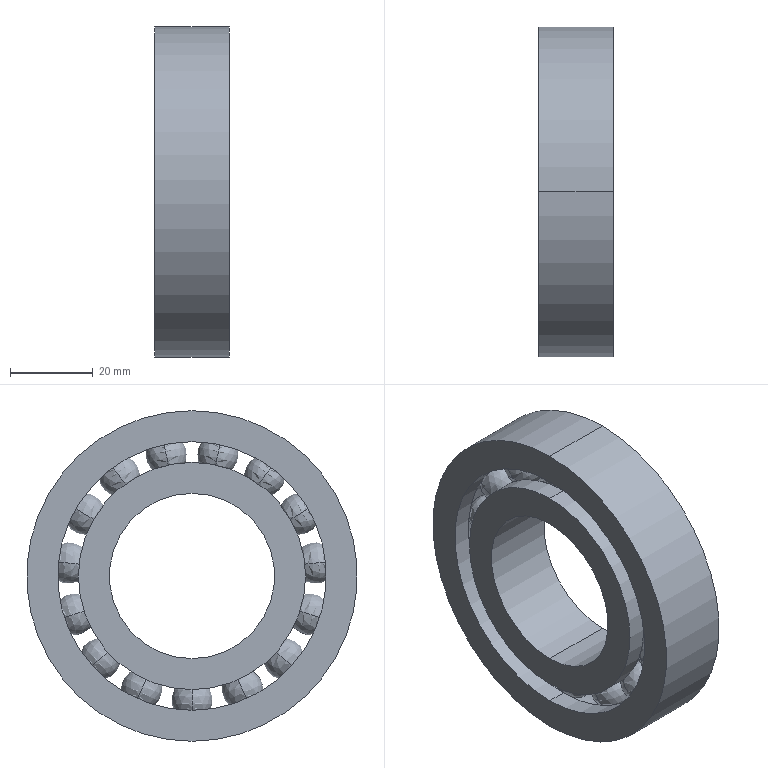Part | NX | features BREP 17 | 17 solids | 50 faces | box 18 x 80 x 80 mm | volume 52959 mm3 | sphere 30 | cylinder 12 | plane 4 | torus 4 | commonest cylinder face diameters 55 x4 65 x4 40 x2 80 x2
STEP:
#1=CARTESIAN_POINT('',(0.,14.695,20.225));
#2=VERTEX_POINT('',#1);
#3=CARTESIAN_POINT('',(0.,20.572,28.316));
#4=VERTEX_POINT('',#3);
#5=CARTESIAN_POINT('',(0.,17.634,24.271));
#6=DIRECTION('',(0.,0.809,-0.5878));
#7=DIRECTION('',(0.,-0.5878,-0.809));
#8=AXIS2_PLACEMENT_3D('',#5,#6,#7);
#9=CIRCLE('',#8,5.);
#10=EDGE_CURVE('',#2,#4,#9,.T.);
#11=ORIENTED_EDGE('',*,*,#10,.T.);
#12=CARTESIAN_POINT('',(0.,17.634,24.271));
#13=DIRECTION('',(0.,-0.809,0.5878));
#14=DIRECTION('',(0.,-0.5878,-0.809));
#15=AXIS2_PLACEMENT_3D('',#12,#13,#14);
#16=CIRCLE('',#15,5.);
#17=EDGE_CURVE('',#2,#4,#16,.T.);
#18=ORIENTED_EDGE('',*,*,#17,.F.);
#19=EDGE_LOOP('',(#11,#18));
#20=FACE_BOUND('',#19,.T.);
#21=CARTESIAN_POINT('',(0.,17.634,24.271));
#22=DIRECTION('',(0.,0.5878,0.809));
#23=DIRECTION('',(-1.,0.,0.));
#24=AXIS2_PLACEMENT_3D('',#21,#22,#23);
#25=SPHERICAL_SURFACE('',#24,5.);
#26=ADVANCED_FACE('',(#20),#25,.T.);
#27=ORIENTED_EDGE('',*,*,#10,.F.);
#28=ORIENTED_EDGE('',*,*,#17,.T.);
#29=EDGE_LOOP('',(#27,#28));
#30=FACE_BOUND('',#29,.T.);
#31=CARTESIAN_POINT('',(0.,17.634,24.271));
#32=DIRECTION('',(0.,0.5878,0.809));
#33=DIRECTION('',(-1.,0.,0.));
#34=AXIS2_PLACEMENT_3D('',#31,#32,#33);
#35=SPHERICAL_SURFACE('',#34,5.);
#36=ADVANCED_FACE('',(#30),#35,.T.);
#37=CLOSED_SHELL('',(#26,#36));
#38=MANIFOLD_SOLID_BREP('',#37);
#39=CARTESIAN_POINT('',(0.,24.863,2.613));
#40=VERTEX_POINT('',#39);
#41=CARTESIAN_POINT('',(0.,34.808,3.658));
#42=VERTEX_POINT('',#41);
#43=CARTESIAN_POINT('',(0.,29.836,3.136));
#44=DIRECTION('',(0.,0.1045,-0.9945));
#45=DIRECTION('',(0.,-0.9945,-0.1045));
#46=AXIS2_PLACEMENT_3D('',#43,#44,#45);
#47=CIRCLE('',#46,5.);
#48=EDGE_CURVE('',#40,#42,#47,.T.);
#49=ORIENTED_EDGE('',*,*,#48,.T.);
#50=CARTESIAN_POINT('',(0.,29.836,3.136));
#51=DIRECTION('',(0.,-0.1045,0.9945));
#52=DIRECTION('',(0.,-0.9945,-0.1045));
#53=AXIS2_PLACEMENT_3D('',#50,#51,#52);
#54=CIRCLE('',#53,5.);
#55=EDGE_CURVE('',#40,#42,#54,.T.);
#56=ORIENTED_EDGE('',*,*,#55,.F.);
#57=EDGE_LOOP('',(#49,#56));
#58=FACE_BOUND('',#57,.T.);
#59=CARTESIAN_POINT('',(0.,29.836,3.136));
#60=DIRECTION('',(0.,0.9945,0.1045));
#61=DIRECTION('',(-1.,0.,0.));
#62=AXIS2_PLACEMENT_3D('',#59,#60,#61);
#63=SPHERICAL_SURFACE('',#62,5.);
#64=ADVANCED_FACE('',(#58),#63,.T.);
#65=ORIENTED_EDGE('',*,*,#48,.F.);
#66=ORIENTED_EDGE('',*,*,#55,.T.);
#67=EDGE_LOOP('',(#65,#66));
#68=FACE_BOUND('',#67,.T.);
#69=CARTESIAN_POINT('',(0.,29.836,3.136));
#70=DIRECTION('',(0.,0.9945,0.1045));
#71=DIRECTION('',(-1.,0.,0.));
#72=AXIS2_PLACEMENT_3D('',#69,#70,#71);
#73=SPHERICAL_SURFACE('',#72,5.);
#74=ADVANCED_FACE('',(#68),#73,.T.);
#75=CLOSED_SHELL('',(#64,#74));
#76=MANIFOLD_SOLID_BREP('',#75);
#77=CARTESIAN_POINT('',(0.,-23.776,-7.725));
#78=VERTEX_POINT('',#77);
#79=CARTESIAN_POINT('',(0.,-33.287,-10.816));
#80=VERTEX_POINT('',#79);
#81=CARTESIAN_POINT('',(0.,-28.532,-9.271));
#82=DIRECTION('',(0.,-0.309,0.9511));
#83=DIRECTION('',(0.,0.9511,0.309));
#84=AXIS2_PLACEMENT_3D('',#81,#82,#83);
#85=CIRCLE('',#84,5.);
#86=EDGE_CURVE('',#78,#80,#85,.T.);
#87=ORIENTED_EDGE('',*,*,#86,.T.);
#88=CARTESIAN_POINT('',(0.,-28.532,-9.271));
#89=DIRECTION('',(0.,0.309,-0.9511));
#90=DIRECTION('',(0.,0.9511,0.309));
#91=AXIS2_PLACEMENT_3D('',#88,#89,#90);
#92=CIRCLE('',#91,5.);
#93=EDGE_CURVE('',#78,#80,#92,.T.);
#94=ORIENTED_EDGE('',*,*,#93,.F.);
#95=EDGE_LOOP('',(#87,#94));
#96=FACE_BOUND('',#95,.T.);
#97=CARTESIAN_POINT('',(0.,-28.532,-9.271));
#98=DIRECTION('',(0.,-0.9511,-0.309));
#99=DIRECTION('',(-1.,0.,0.));
#100=AXIS2_PLACEMENT_3D('',#97,#98,#99);
#101=SPHERICAL_SURFACE('',#100,5.);
#102=ADVANCED_FACE('',(#96),#101,.T.);
#103=ORIENTED_EDGE('',*,*,#86,.F.);
#104=ORIENTED_EDGE('',*,*,#93,.T.);
#105=EDGE_LOOP('',(#103,#104));
#106=FACE_BOUND('',#105,.T.);
#107=CARTESIAN_POINT('',(0.,-28.532,-9.271));
#108=DIRECTION('',(0.,-0.9511,-0.309));
#109=DIRECTION('',(-1.,0.,0.));
#110=AXIS2_PLACEMENT_3D('',#107,#108,#109);
#111=SPHERICAL_SURFACE('',#110,5.);
#112=ADVANCED_FACE('',(#106),#111,.T.);
#113=CLOSED_SHELL('',(#102,#112));
#114=MANIFOLD_SOLID_BREP('',#113);
#115=CARTESIAN_POINT('',(0.,-10.168,-22.839));
#116=VERTEX_POINT('',#115);
#117=CARTESIAN_POINT('',(0.,-14.236,-31.974));
#118=VERTEX_POINT('',#117);
#119=CARTESIAN_POINT('',(0.,-12.202,-27.406));
#120=DIRECTION('',(0.,-0.9135,0.4067));
#121=DIRECTION('',(0.,0.4067,0.9135));
#122=AXIS2_PLACEMENT_3D('',#119,#120,#121);
#123=CIRCLE('',#122,5.);
#124=EDGE_CURVE('',#116,#118,#123,.T.);
#125=ORIENTED_EDGE('',*,*,#124,.T.);
#126=CARTESIAN_POINT('',(0.,-12.202,-27.406));
#127=DIRECTION('',(0.,0.9135,-0.4067));
#128=DIRECTION('',(0.,0.4067,0.9135));
#129=AXIS2_PLACEMENT_3D('',#126,#127,#128);
#130=CIRCLE('',#129,5.);
#131=EDGE_CURVE('',#116,#118,#130,.T.);
#132=ORIENTED_EDGE('',*,*,#131,.F.);
#133=EDGE_LOOP('',(#125,#132));
#134=FACE_BOUND('',#133,.T.);
#135=CARTESIAN_POINT('',(0.,-12.202,-27.406));
#136=DIRECTION('',(0.,-0.4067,-0.9135));
#137=DIRECTION('',(-1.,0.,0.));
#138=AXIS2_PLACEMENT_3D('',#135,#136,#137);
#139=SPHERICAL_SURFACE('',#138,5.);
#140=ADVANCED_FACE('',(#134),#139,.T.);
#141=ORIENTED_EDGE('',*,*,#124,.F.);
#142=ORIENTED_EDGE('',*,*,#131,.T.);
#143=EDGE_LOOP('',(#141,#142));
#144=FACE_BOUND('',#143,.T.);
#145=CARTESIAN_POINT('',(0.,-12.202,-27.406));
#146=DIRECTION('',(0.,-0.4067,-0.9135));
#147=DIRECTION('',(-1.,0.,0.));
#148=AXIS2_PLACEMENT_3D('',#145,#146,#147);
#149=SPHERICAL_SURFACE('',#148,5.);
#150=ADVANCED_FACE('',(#144),#149,.T.);
#151=CLOSED_SHELL('',(#140,#150));
#152=MANIFOLD_SOLID_BREP('',#151);
#153=CARTESIAN_POINT('',(0.,-5.198,24.454));
#154=VERTEX_POINT('',#153);
#155=CARTESIAN_POINT('',(0.,-7.277,34.235));
#156=VERTEX_POINT('',#155);
#157=CARTESIAN_POINT('',(0.,-6.237,29.344));
#158=DIRECTION('',(0.,0.9781,0.2079));
#159=DIRECTION('',(0.,0.2079,-0.9781));
#160=AXIS2_PLACEMENT_3D('',#157,#158,#159);
#161=CIRCLE('',#160,5.);
#162=EDGE_CURVE('',#154,#156,#161,.T.);
#163=ORIENTED_EDGE('',*,*,#162,.T.);
#164=CARTESIAN_POINT('',(0.,-6.237,29.344));
#165=DIRECTION('',(0.,-0.9781,-0.2079));
#166=DIRECTION('',(0.,0.2079,-0.9781));
#167=AXIS2_PLACEMENT_3D('',#164,#165,#166);
#168=CIRCLE('',#167,5.);
#169=EDGE_CURVE('',#154,#156,#168,.T.);
#170=ORIENTED_EDGE('',*,*,#169,.F.);
#171=EDGE_LOOP('',(#163,#170));
#172=FACE_BOUND('',#171,.T.);
#173=CARTESIAN_POINT('',(0.,-6.237,29.344));
#174=DIRECTION('',(0.,-0.2079,0.9781));
#175=DIRECTION('',(-1.,0.,0.));
#176=AXIS2_PLACEMENT_3D('',#173,#174,#175);
#177=SPHERICAL_SURFACE('',#176,5.);
#178=ADVANCED_FACE('',(#172),#177,.T.);
#179=ORIENTED_EDGE('',*,*,#162,.F.);
#180=ORIENTED_EDGE('',*,*,#169,.T.);
#181=EDGE_LOOP('',(#179,#180));
#182=FACE_BOUND('',#181,.T.);
#183=CARTESIAN_POINT('',(0.,-6.237,29.344));
#184=DIRECTION('',(0.,-0.2079,0.9781));
#185=DIRECTION('',(-1.,0.,0.));
#186=AXIS2_PLACEMENT_3D('',#183,#184,#185);
#187=SPHERICAL_SURFACE('',#186,5.);
#188=ADVANCED_FACE('',(#182),#187,.T.);
#189=CLOSED_SHELL('',(#178,#188));
#190=MANIFOLD_SOLID_BREP('',#189);
#191=CARTESIAN_POINT('',(-9.,0.,-40.));
#192=VERTEX_POINT('',#191);
#193=CARTESIAN_POINT('',(-9.,0.,40.));
#194=VERTEX_POINT('',#193);
#195=CARTESIAN_POINT('',(-9.,0.,0.));
#196=DIRECTION('',(1.,0.,0.));
#197=DIRECTION('',(0.,0.,-1.));
#198=AXIS2_PLACEMENT_3D('',#195,#196,#197);
#199=CIRCLE('',#198,40.);
#200=EDGE_CURVE('',#192,#194,#199,.T.);
#201=ORIENTED_EDGE('',*,*,#200,.T.);
#202=CARTESIAN_POINT('',(9.,0.,40.));
#203=VERTEX_POINT('',#202);
#204=CARTESIAN_POINT('',(9.,0.,40.));
#205=DIRECTION('',(-1.,0.,0.));
#206=VECTOR('',#205,1000.);
#207=LINE('',#204,#206);
#208=EDGE_CURVE('',#203,#194,#207,.T.);
#209=ORIENTED_EDGE('',*,*,#208,.F.);
#210=CARTESIAN_POINT('',(9.,0.,-40.));
#211=VERTEX_POINT('',#210);
#212=CARTESIAN_POINT('',(9.,0.,0.));
#213=DIRECTION('',(1.,0.,0.));
#214=DIRECTION('',(0.,0.,-1.));
#215=AXIS2_PLACEMENT_3D('',#212,#213,#214);
#216=CIRCLE('',#215,40.);
#217=EDGE_CURVE('',#211,#203,#216,.T.);
#218=ORIENTED_EDGE('',*,*,#217,.F.);
#219=CARTESIAN_POINT('',(9.,0.,-40.));
#220=DIRECTION('',(-1.,0.,0.));
#221=VECTOR('',#220,1000.);
#222=LINE('',#219,#221);
#223=EDGE_CURVE('',#211,#192,#222,.T.);
#224=ORIENTED_EDGE('',*,*,#223,.T.);
#225=EDGE_LOOP('',(#201,#209,#218,#224));
#226=FACE_BOUND('',#225,.T.);
#227=CARTESIAN_POINT('',(9.9,0.,0.));
#228=DIRECTION('',(-1.,0.,0.));
#229=DIRECTION('',(0.,0.,1.));
#230=AXIS2_PLACEMENT_3D('',#227,#228,#229);
#231=CYLINDRICAL_SURFACE('',#230,40.);
#232=ADVANCED_FACE('',(#226),#231,.T.);
#233=CARTESIAN_POINT('',(9.,0.,0.));
#234=DIRECTION('',(-1.,0.,0.));
#235=DIRECTION('',(0.,0.,-1.));
#236=AXIS2_PLACEMENT_3D('',#233,#234,#235);
#237=CIRCLE('',#236,40.);
#238=EDGE_CURVE('',#211,#203,#237,.T.);
#239=ORIENTED_EDGE('',*,*,#238,.T.);
#240=ORIENTED_EDGE('',*,*,#208,.T.);
#241=CARTESIAN_POINT('',(-9.,0.,0.));
#242=DIRECTION('',(-1.,0.,0.));
#243=DIRECTION('',(0.,0.,-1.));
#244=AXIS2_PLACEMENT_3D('',#241,#242,#243);
#245=CIRCLE('',#244,40.);
#246=EDGE_CURVE('',#192,#194,#245,.T.);
#247=ORIENTED_EDGE('',*,*,#246,.F.);
#248=ORIENTED_EDGE('',*,*,#223,.F.);
#249=EDGE_LOOP('',(#239,#240,#247,#248));
#250=FACE_BOUND('',#249,.T.);
#251=CARTESIAN_POINT('',(9.9,0.,0.));
#252=DIRECTION('',(-1.,0.,0.));
#253=DIRECTION('',(0.,0.,1.));
#254=AXIS2_PLACEMENT_3D('',#251,#252,#253);
#255=CYLINDRICAL_SURFACE('',#254,40.);
#256=ADVANCED_FACE('',(#250),#255,.T.);
#257=ORIENTED_EDGE('',*,*,#200,.F.);
#258=ORIENTED_EDGE('',*,*,#246,.T.);
#259=EDGE_LOOP('',(#257,#258));
#260=FACE_BOUND('',#259,.T.);
#261=CARTESIAN_POINT('',(-9.,0.,-32.5));
#262=VERTEX_POINT('',#261);
#263=CARTESIAN_POINT('',(-9.,0.,32.5));
#264=VERTEX_POINT('',#263);
#265=CARTESIAN_POINT('',(-9.,0.,0.));
#266=DIRECTION('',(-1.,0.,0.));
#267=DIRECTION('',(0.,0.,-1.));
#268=AXIS2_PLACEMENT_3D('',#265,#266,#267);
#269=CIRCLE('',#268,32.5);
#270=EDGE_CURVE('',#262,#264,#269,.T.);
#271=ORIENTED_EDGE('',*,*,#270,.F.);
#272=CARTESIAN_POINT('',(-9.,0.,0.));
#273=DIRECTION('',(1.,0.,0.));
#274=DIRECTION('',(0.,0.,-1.));
#275=AXIS2_PLACEMENT_3D('',#272,#273,#274);
#276=CIRCLE('',#275,32.5);
#277=EDGE_CURVE('',#262,#264,#276,.T.);
#278=ORIENTED_EDGE('',*,*,#277,.T.);
#279=EDGE_LOOP('',(#271,#278));
#280=FACE_BOUND('',#279,.T.);
#281=CARTESIAN_POINT('',(-9.,0.,0.));
#282=DIRECTION('',(-1.,0.,0.));
#283=DIRECTION('',(0.,0.,1.));
#284=AXIS2_PLACEMENT_3D('',#281,#282,#283);
#285=PLANE('',#284);
#286=ADVANCED_FACE('',(#260,#280),#285,.T.);
#287=CARTESIAN_POINT('',(-4.33,0.,-32.5));
#288=VERTEX_POINT('',#287);
#289=CARTESIAN_POINT('',(-4.33,0.,32.5));
#290=VERTEX_POINT('',#289);
#291=CARTESIAN_POINT('',(-4.33,0.,0.));
#292=DIRECTION('',(1.,0.,0.));
#293=DIRECTION('',(0.,0.,-1.));
#294=AXIS2_PLACEMENT_3D('',#291,#292,#293);
#295=CIRCLE('',#294,32.5);
#296=EDGE_CURVE('',#288,#290,#295,.T.);
#297=ORIENTED_EDGE('',*,*,#296,.T.);
#298=CARTESIAN_POINT('',(-9.,0.,32.5));
#299=DIRECTION('',(1.,0.,0.));
#300=VECTOR('',#299,1000.);
#301=LINE('',#298,#300);
#302=EDGE_CURVE('',#264,#290,#301,.T.);
#303=ORIENTED_EDGE('',*,*,#302,.F.);
#304=ORIENTED_EDGE('',*,*,#277,.F.);
#305=CARTESIAN_POINT('',(-9.,0.,-32.5));
#306=DIRECTION('',(1.,0.,0.));
#307=VECTOR('',#306,1000.);
#308=LINE('',#305,#307);
#309=EDGE_CURVE('',#262,#288,#308,.T.);
#310=ORIENTED_EDGE('',*,*,#309,.T.);
#311=EDGE_LOOP('',(#297,#303,#304,#310));
#312=FACE_BOUND('',#311,.T.);
#313=CARTESIAN_POINT('',(9.9,0.,0.));
#314=DIRECTION('',(-1.,0.,0.));
#315=DIRECTION('',(0.,0.,1.));
#316=AXIS2_PLACEMENT_3D('',#313,#314,#315);
#317=CYLINDRICAL_SURFACE('',#316,32.5);
#318=ADVANCED_FACE('',(#312),#317,.F.);
#319=ORIENTED_EDGE('',*,*,#270,.T.);
#320=ORIENTED_EDGE('',*,*,#302,.T.);
#321=CARTESIAN_POINT('',(-4.33,0.,0.));
#322=DIRECTION('',(-1.,0.,0.));
#323=DIRECTION('',(0.,0.,-1.));
#324=AXIS2_PLACEMENT_3D('',#321,#322,#323);
#325=CIRCLE('',#324,32.5);
#326=EDGE_CURVE('',#288,#290,#325,.T.);
#327=ORIENTED_EDGE('',*,*,#326,.F.);
#328=ORIENTED_EDGE('',*,*,#309,.F.);
#329=EDGE_LOOP('',(#319,#320,#327,#328));
#330=FACE_BOUND('',#329,.T.);
#331=CARTESIAN_POINT('',(9.9,0.,0.));
#332=DIRECTION('',(-1.,0.,0.));
#333=DIRECTION('',(0.,0.,1.));
#334=AXIS2_PLACEMENT_3D('',#331,#332,#333);
#335=CYLINDRICAL_SURFACE('',#334,32.5);
#336=ADVANCED_FACE('',(#330),#335,.F.);
#337=ORIENTED_EDGE('',*,*,#326,.T.);
#338=CARTESIAN_POINT('',(4.33,0.,32.5));
#339=VERTEX_POINT('',#338);
#340=CARTESIAN_POINT('',(0.,0.,30.));
#341=DIRECTION('',(0.,1.,0.));
#342=DIRECTION('',(-0.866,0.,0.5));
#343=AXIS2_PLACEMENT_3D('',#340,#341,#342);
#344=CIRCLE('',#343,5.);
#345=EDGE_CURVE('',#339,#290,#344,.F.);
#346=ORIENTED_EDGE('',*,*,#345,.F.);
#347=CARTESIAN_POINT('',(4.33,0.,-32.5));
#348=VERTEX_POINT('',#347);
#349=CARTESIAN_POINT('',(4.33,0.,0.));
#350=DIRECTION('',(-1.,0.,0.));
#351=DIRECTION('',(0.,0.,-1.));
#352=AXIS2_PLACEMENT_3D('',#349,#350,#351);
#353=CIRCLE('',#352,32.5);
#354=EDGE_CURVE('',#348,#339,#353,.T.);
#355=ORIENTED_EDGE('',*,*,#354,.F.);
#356=CARTESIAN_POINT('',(0.,0.,-30.));
#357=DIRECTION('',(0.,-1.,0.));
#358=DIRECTION('',(-0.866,0.,-0.5));
#359=AXIS2_PLACEMENT_3D('',#356,#357,#358);
#360=CIRCLE('',#359,5.);
#361=EDGE_CURVE('',#348,#288,#360,.F.);
#362=ORIENTED_EDGE('',*,*,#361,.T.);
#363=EDGE_LOOP('',(#337,#346,#355,#362));
#364=FACE_BOUND('',#363,.T.);
#365=CARTESIAN_POINT('',(0.,0.,0.));
#366=DIRECTION('',(-1.,0.,0.));
#367=DIRECTION('',(0.,0.,1.));
#368=AXIS2_PLACEMENT_3D('',#365,#366,#367);
#369=TOROIDAL_SURFACE('',#368,30.,5.);
#370=ADVANCED_FACE('',(#364),#369,.F.);
#371=CARTESIAN_POINT('',(4.33,0.,0.));
#372=DIRECTION('',(1.,0.,0.));
#373=DIRECTION('',(0.,0.,-1.));
#374=AXIS2_PLACEMENT_3D('',#371,#372,#373);
#375=CIRCLE('',#374,32.5);
#376=EDGE_CURVE('',#348,#339,#375,.T.);
#377=ORIENTED_EDGE('',*,*,#376,.T.);
#378=ORIENTED_EDGE('',*,*,#345,.T.);
#379=ORIENTED_EDGE('',*,*,#296,.F.);
#380=ORIENTED_EDGE('',*,*,#361,.F.);
#381=EDGE_LOOP('',(#377,#378,#379,#380));
#382=FACE_BOUND('',#381,.T.);
#383=CARTESIAN_POINT('',(0.,0.,0.));
#384=DIRECTION('',(-1.,0.,0.));
#385=DIRECTION('',(0.,0.,1.));
#386=AXIS2_PLACEMENT_3D('',#383,#384,#385);
#387=TOROIDAL_SURFACE('',#386,30.,5.);
#388=ADVANCED_FACE('',(#382),#387,.F.);
#389=CARTESIAN_POINT('',(9.,0.,-32.5));
#390=VERTEX_POINT('',#389);
#391=CARTESIAN_POINT('',(9.,0.,32.5));
#392=VERTEX_POINT('',#391);
#393=CARTESIAN_POINT('',(9.,0.,0.));
#394=DIRECTION('',(1.,0.,0.));
#395=DIRECTION('',(0.,0.,-1.));
#396=AXIS2_PLACEMENT_3D('',#393,#394,#395);
#397=CIRCLE('',#396,32.5);
#398=EDGE_CURVE('',#390,#392,#397,.T.);
#399=ORIENTED_EDGE('',*,*,#398,.T.);
#400=CARTESIAN_POINT('',(4.33,0.,32.5));
#401=DIRECTION('',(1.,0.,0.));
#402=VECTOR('',#401,1000.);
#403=LINE('',#400,#402);
#404=EDGE_CURVE('',#339,#392,#403,.T.);
#405=ORIENTED_EDGE('',*,*,#404,.F.);
#406=ORIENTED_EDGE('',*,*,#376,.F.);
#407=CARTESIAN_POINT('',(4.33,0.,-32.5));
#408=DIRECTION('',(1.,0.,0.));
#409=VECTOR('',#408,1000.);
#410=LINE('',#407,#409);
#411=EDGE_CURVE('',#348,#390,#410,.T.);
#412=ORIENTED_EDGE('',*,*,#411,.T.);
#413=EDGE_LOOP('',(#399,#405,#406,#412));
#414=FACE_BOUND('',#413,.T.);
#415=CARTESIAN_POINT('',(9.9,0.,0.));
#416=DIRECTION('',(-1.,0.,0.));
#417=DIRECTION('',(0.,0.,1.));
#418=AXIS2_PLACEMENT_3D('',#415,#416,#417);
#419=CYLINDRICAL_SURFACE('',#418,32.5);
#420=ADVANCED_FACE('',(#414),#419,.F.);
#421=ORIENTED_EDGE('',*,*,#354,.T.);
#422=ORIENTED_EDGE('',*,*,#404,.T.);
#423=CARTESIAN_POINT('',(9.,0.,0.));
#424=DIRECTION('',(-1.,0.,0.));
#425=DIRECTION('',(0.,0.,-1.));
#426=AXIS2_PLACEMENT_3D('',#423,#424,#425);
#427=CIRCLE('',#426,32.5);
#428=EDGE_CURVE('',#390,#392,#427,.T.);
#429=ORIENTED_EDGE('',*,*,#428,.F.);
#430=ORIENTED_EDGE('',*,*,#411,.F.);
#431=EDGE_LOOP('',(#421,#422,#429,#430));
#432=FACE_BOUND('',#431,.T.);
#433=CARTESIAN_POINT('',(9.9,0.,0.));
#434=DIRECTION('',(-1.,0.,0.));
#435=DIRECTION('',(0.,0.,1.));
#436=AXIS2_PLACEMENT_3D('',#433,#434,#435);
#437=CYLINDRICAL_SURFACE('',#436,32.5);
#438=ADVANCED_FACE('',(#432),#437,.F.);
#439=ORIENTED_EDGE('',*,*,#238,.F.);
#440=ORIENTED_EDGE('',*,*,#217,.T.);
#441=EDGE_LOOP('',(#439,#440));
#442=FACE_BOUND('',#441,.T.);
#443=ORIENTED_EDGE('',*,*,#398,.F.);
#444=ORIENTED_EDGE('',*,*,#428,.T.);
#445=EDGE_LOOP('',(#443,#444));
#446=FACE_BOUND('',#445,.T.);
#447=CARTESIAN_POINT('',(9.,0.,0.));
#448=DIRECTION('',(-1.,0.,0.));
#449=DIRECTION('',(0.,0.,1.));
#450=AXIS2_PLACEMENT_3D('',#447,#448,#449);
#451=PLANE('',#450);
#452=ADVANCED_FACE('',(#442,#446),#451,.F.);
#453=CLOSED_SHELL('',(#232,#256,#286,#318,#336,#370,#388,#420,#438,#452));
#454=MANIFOLD_SOLID_BREP('',#453);
#455=CARTESIAN_POINT('',(0.,23.776,-7.725));
#456=VERTEX_POINT('',#455);
#457=CARTESIAN_POINT('',(0.,33.287,-10.816));
#458=VERTEX_POINT('',#457);
#459=CARTESIAN_POINT('',(0.,28.532,-9.271));
#460=DIRECTION('',(0.,-0.309,-0.9511));
#461=DIRECTION('',(0.,-0.9511,0.309));
#462=AXIS2_PLACEMENT_3D('',#459,#460,#461);
#463=CIRCLE('',#462,5.);
#464=EDGE_CURVE('',#456,#458,#463,.T.);
#465=ORIENTED_EDGE('',*,*,#464,.T.);
#466=CARTESIAN_POINT('',(0.,28.532,-9.271));
#467=DIRECTION('',(0.,0.309,0.9511));
#468=DIRECTION('',(0.,-0.9511,0.309));
#469=AXIS2_PLACEMENT_3D('',#466,#467,#468);
#470=CIRCLE('',#469,5.);
#471=EDGE_CURVE('',#456,#458,#470,.T.);
#472=ORIENTED_EDGE('',*,*,#471,.F.);
#473=EDGE_LOOP('',(#465,#472));
#474=FACE_BOUND('',#473,.T.);
#475=CARTESIAN_POINT('',(0.,28.532,-9.271));
#476=DIRECTION('',(0.,0.9511,-0.309));
#477=DIRECTION('',(-1.,0.,0.));
#478=AXIS2_PLACEMENT_3D('',#475,#476,#477);
#479=SPHERICAL_SURFACE('',#478,5.);
#480=ADVANCED_FACE('',(#474),#479,.T.);
#481=ORIENTED_EDGE('',*,*,#464,.F.);
#482=ORIENTED_EDGE('',*,*,#471,.T.);
#483=EDGE_LOOP('',(#481,#482));
#484=FACE_BOUND('',#483,.T.);
#485=CARTESIAN_POINT('',(0.,28.532,-9.271));
#486=DIRECTION('',(0.,0.9511,-0.309));
#487=DIRECTION('',(-1.,0.,0.));
#488=AXIS2_PLACEMENT_3D('',#485,#486,#487);
#489=SPHERICAL_SURFACE('',#488,5.);
#490=ADVANCED_FACE('',(#484),#489,.T.);
#491=CLOSED_SHELL('',(#480,#490));
#492=MANIFOLD_SOLID_BREP('',#491);
#493=CARTESIAN_POINT('',(0.,-14.695,20.225));
#494=VERTEX_POINT('',#493);
#495=CARTESIAN_POINT('',(0.,-20.572,28.316));
#496=VERTEX_POINT('',#495);
#497=CARTESIAN_POINT('',(0.,-17.634,24.271));
#498=DIRECTION('',(0.,0.809,0.5878));
#499=DIRECTION('',(0.,0.5878,-0.809));
#500=AXIS2_PLACEMENT_3D('',#497,#498,#499);
#501=CIRCLE('',#500,5.);
#502=EDGE_CURVE('',#494,#496,#501,.T.);
#503=ORIENTED_EDGE('',*,*,#502,.T.);
#504=CARTESIAN_POINT('',(0.,-17.634,24.271));
#505=DIRECTION('',(0.,-0.809,-0.5878));
#506=DIRECTION('',(0.,0.5878,-0.809));
#507=AXIS2_PLACEMENT_3D('',#504,#505,#506);
#508=CIRCLE('',#507,5.);
#509=EDGE_CURVE('',#494,#496,#508,.T.);
#510=ORIENTED_EDGE('',*,*,#509,.F.);
#511=EDGE_LOOP('',(#503,#510));
#512=FACE_BOUND('',#511,.T.);
#513=CARTESIAN_POINT('',(0.,-17.634,24.271));
#514=DIRECTION('',(0.,-0.5878,0.809));
#515=DIRECTION('',(-1.,0.,0.));
#516=AXIS2_PLACEMENT_3D('',#513,#514,#515);
#517=SPHERICAL_SURFACE('',#516,5.);
#518=ADVANCED_FACE('',(#512),#517,.T.);
#519=ORIENTED_EDGE('',*,*,#502,.F.);
#520=ORIENTED_EDGE('',*,*,#509,.T.);
#521=EDGE_LOOP('',(#519,#520));
#522=FACE_BOUND('',#521,.T.);
#523=CARTESIAN_POINT('',(0.,-17.634,24.271));
#524=DIRECTION('',(0.,-0.5878,0.809));
#525=DIRECTION('',(-1.,0.,0.));
#526=AXIS2_PLACEMENT_3D('',#523,#524,#525);
#527=SPHERICAL_SURFACE('',#526,5.);
#528=ADVANCED_FACE('',(#522),#527,.T.);
#529=CLOSED_SHELL('',(#518,#528));
#530=MANIFOLD_SOLID_BREP('',#529);
#531=CARTESIAN_POINT('',(0.,-18.579,-16.728));
#532=VERTEX_POINT('',#531);
#533=CARTESIAN_POINT('',(0.,-26.01,-23.42));
#534=VERTEX_POINT('',#533);
#535=CARTESIAN_POINT('',(0.,-22.294,-20.074));
#536=DIRECTION('',(0.,-0.6691,0.7431));
#537=DIRECTION('',(0.,0.7431,0.6691));
#538=AXIS2_PLACEMENT_3D('',#535,#536,#537);
#539=CIRCLE('',#538,5.);
#540=EDGE_CURVE('',#532,#534,#539,.T.);
#541=ORIENTED_EDGE('',*,*,#540,.T.);
#542=CARTESIAN_POINT('',(0.,-22.294,-20.074));
#543=DIRECTION('',(0.,0.6691,-0.7431));
#544=DIRECTION('',(0.,0.7431,0.6691));
#545=AXIS2_PLACEMENT_3D('',#542,#543,#544);
#546=CIRCLE('',#545,5.);
#547=EDGE_CURVE('',#532,#534,#546,.T.);
#548=ORIENTED_EDGE('',*,*,#547,.F.);
#549=EDGE_LOOP('',(#541,#548));
#550=FACE_BOUND('',#549,.T.);
#551=CARTESIAN_POINT('',(0.,-22.294,-20.074));
#552=DIRECTION('',(0.,-0.7431,-0.6691));
#553=DIRECTION('',(-1.,0.,0.));
#554=AXIS2_PLACEMENT_3D('',#551,#552,#553);
#555=SPHERICAL_SURFACE('',#554,5.);
#556=ADVANCED_FACE('',(#550),#555,.T.);
#557=ORIENTED_EDGE('',*,*,#540,.F.);
#558=ORIENTED_EDGE('',*,*,#547,.T.);
#559=EDGE_LOOP('',(#557,#558));
#560=FACE_BOUND('',#559,.T.);
#561=CARTESIAN_POINT('',(0.,-22.294,-20.074));
#562=DIRECTION('',(0.,-0.7431,-0.6691));
#563=DIRECTION('',(-1.,0.,0.));
#564=AXIS2_PLACEMENT_3D('',#561,#562,#563);
#565=SPHERICAL_SURFACE('',#564,5.);
#566=ADVANCED_FACE('',(#560),#565,.T.);
#567=CLOSED_SHELL('',(#556,#566));
#568=MANIFOLD_SOLID_BREP('',#567);
#569=CARTESIAN_POINT('',(0.,21.651,12.5));
#570=VERTEX_POINT('',#569);
#571=CARTESIAN_POINT('',(0.,30.311,17.5));
#572=VERTEX_POINT('',#571);
#573=CARTESIAN_POINT('',(0.,25.981,15.));
#574=DIRECTION('',(0.,0.5,-0.866));
#575=DIRECTION('',(0.,-0.866,-0.5));
#576=AXIS2_PLACEMENT_3D('',#573,#574,#575);
#577=CIRCLE('',#576,5.);
#578=EDGE_CURVE('',#570,#572,#577,.T.);
#579=ORIENTED_EDGE('',*,*,#578,.T.);
#580=CARTESIAN_POINT('',(0.,25.981,15.));
#581=DIRECTION('',(0.,-0.5,0.866));
#582=DIRECTION('',(0.,-0.866,-0.5));
#583=AXIS2_PLACEMENT_3D('',#580,#581,#582);
#584=CIRCLE('',#583,5.);
#585=EDGE_CURVE('',#570,#572,#584,.T.);
#586=ORIENTED_EDGE('',*,*,#585,.F.);
#587=EDGE_LOOP('',(#579,#586));
#588=FACE_BOUND('',#587,.T.);
#589=CARTESIAN_POINT('',(0.,25.981,15.));
#590=DIRECTION('',(0.,0.866,0.5));
#591=DIRECTION('',(-1.,0.,0.));
#592=AXIS2_PLACEMENT_3D('',#589,#590,#591);
#593=SPHERICAL_SURFACE('',#592,5.);
#594=ADVANCED_FACE('',(#588),#593,.T.);
#595=ORIENTED_EDGE('',*,*,#578,.F.);
#596=ORIENTED_EDGE('',*,*,#585,.T.);
#597=EDGE_LOOP('',(#595,#596));
#598=FACE_BOUND('',#597,.T.);
#599=CARTESIAN_POINT('',(0.,25.981,15.));
#600=DIRECTION('',(0.,0.866,0.5));
#601=DIRECTION('',(-1.,0.,0.));
#602=AXIS2_PLACEMENT_3D('',#599,#600,#601);
#603=SPHERICAL_SURFACE('',#602,5.);
#604=ADVANCED_FACE('',(#598),#603,.T.);
#605=CLOSED_SHELL('',(#594,#604));
#606=MANIFOLD_SOLID_BREP('',#605);
#607=CARTESIAN_POINT('',(0.,-24.863,2.613));
#608=VERTEX_POINT('',#607);
#609=CARTESIAN_POINT('',(0.,-34.808,3.658));
#610=VERTEX_POINT('',#609);
#611=CARTESIAN_POINT('',(0.,-29.836,3.136));
#612=DIRECTION('',(0.,0.1045,0.9945));
#613=DIRECTION('',(0.,0.9945,-0.1045));
#614=AXIS2_PLACEMENT_3D('',#611,#612,#613);
#615=CIRCLE('',#614,5.);
#616=EDGE_CURVE('',#608,#610,#615,.T.);
#617=ORIENTED_EDGE('',*,*,#616,.T.);
#618=CARTESIAN_POINT('',(0.,-29.836,3.136));
#619=DIRECTION('',(0.,-0.1045,-0.9945));
#620=DIRECTION('',(0.,0.9945,-0.1045));
#621=AXIS2_PLACEMENT_3D('',#618,#619,#620);
#622=CIRCLE('',#621,5.);
#623=EDGE_CURVE('',#608,#610,#622,.T.);
#624=ORIENTED_EDGE('',*,*,#623,.F.);
#625=EDGE_LOOP('',(#617,#624));
#626=FACE_BOUND('',#625,.T.);
#627=CARTESIAN_POINT('',(0.,-29.836,3.136));
#628=DIRECTION('',(0.,-0.9945,0.1045));
#629=DIRECTION('',(-1.,0.,0.));
#630=AXIS2_PLACEMENT_3D('',#627,#628,#629);
#631=SPHERICAL_SURFACE('',#630,5.);
#632=ADVANCED_FACE('',(#626),#631,.T.);
#633=ORIENTED_EDGE('',*,*,#616,.F.);
#634=ORIENTED_EDGE('',*,*,#623,.T.);
#635=EDGE_LOOP('',(#633,#634));
#636=FACE_BOUND('',#635,.T.);
#637=CARTESIAN_POINT('',(0.,-29.836,3.136));
#638=DIRECTION('',(0.,-0.9945,0.1045));
#639=DIRECTION('',(-1.,0.,0.));
#640=AXIS2_PLACEMENT_3D('',#637,#638,#639);
#641=SPHERICAL_SURFACE('',#640,5.);
#642=ADVANCED_FACE('',(#636),#641,.T.);
#643=CLOSED_SHELL('',(#632,#642));
#644=MANIFOLD_SOLID_BREP('',#643);
#645=CARTESIAN_POINT('',(0.,10.168,-22.839));
#646=VERTEX_POINT('',#645);
#647=CARTESIAN_POINT('',(0.,14.236,-31.974));
#648=VERTEX_POINT('',#647);
#649=CARTESIAN_POINT('',(0.,12.202,-27.406));
#650=DIRECTION('',(0.,-0.9135,-0.4067));
#651=DIRECTION('',(0.,-0.4067,0.9135));
#652=AXIS2_PLACEMENT_3D('',#649,#650,#651);
#653=CIRCLE('',#652,5.);
#654=EDGE_CURVE('',#646,#648,#653,.T.);
#655=ORIENTED_EDGE('',*,*,#654,.T.);
#656=CARTESIAN_POINT('',(0.,12.202,-27.406));
#657=DIRECTION('',(0.,0.9135,0.4067));
#658=DIRECTION('',(0.,-0.4067,0.9135));
#659=AXIS2_PLACEMENT_3D('',#656,#657,#658);
#660=CIRCLE('',#659,5.);
#661=EDGE_CURVE('',#646,#648,#660,.T.);
#662=ORIENTED_EDGE('',*,*,#661,.F.);
#663=EDGE_LOOP('',(#655,#662));
#664=FACE_BOUND('',#663,.T.);
#665=CARTESIAN_POINT('',(0.,12.202,-27.406));
#666=DIRECTION('',(0.,0.4067,-0.9135));
#667=DIRECTION('',(-1.,0.,0.));
#668=AXIS2_PLACEMENT_3D('',#665,#666,#667);
#669=SPHERICAL_SURFACE('',#668,5.);
#670=ADVANCED_FACE('',(#664),#669,.T.);
#671=ORIENTED_EDGE('',*,*,#654,.F.);
#672=ORIENTED_EDGE('',*,*,#661,.T.);
#673=EDGE_LOOP('',(#671,#672));
#674=FACE_BOUND('',#673,.T.);
#675=CARTESIAN_POINT('',(0.,12.202,-27.406));
#676=DIRECTION('',(0.,0.4067,-0.9135));
#677=DIRECTION('',(-1.,0.,0.));
#678=AXIS2_PLACEMENT_3D('',#675,#676,#677);
#679=SPHERICAL_SURFACE('',#678,5.);
#680=ADVANCED_FACE('',(#674),#679,.T.);
#681=CLOSED_SHELL('',(#670,#680));
#682=MANIFOLD_SOLID_BREP('',#681);
#683=CARTESIAN_POINT('',(-9.,0.,-27.5));
#684=VERTEX_POINT('',#683);
#685=CARTESIAN_POINT('',(-9.,0.,27.5));
#686=VERTEX_POINT('',#685);
#687=CARTESIAN_POINT('',(-9.,0.,0.));
#688=DIRECTION('',(1.,0.,0.));
#689=DIRECTION('',(0.,0.,-1.));
#690=AXIS2_PLACEMENT_3D('',#687,#688,#689);
#691=CIRCLE('',#690,27.5);
#692=EDGE_CURVE('',#684,#686,#691,.T.);
#693=ORIENTED_EDGE('',*,*,#692,.T.);
#694=CARTESIAN_POINT('',(-4.33,0.,27.5));
#695=VERTEX_POINT('',#694);
#696=CARTESIAN_POINT('',(-4.33,0.,27.5));
#697=DIRECTION('',(-1.,0.,0.));
#698=VECTOR('',#697,1000.);
#699=LINE('',#696,#698);
#700=EDGE_CURVE('',#695,#686,#699,.T.);
#701=ORIENTED_EDGE('',*,*,#700,.F.);
#702=CARTESIAN_POINT('',(-4.33,0.,-27.5));
#703=VERTEX_POINT('',#702);
#704=CARTESIAN_POINT('',(-4.33,0.,0.));
#705=DIRECTION('',(1.,0.,0.));
#706=DIRECTION('',(0.,0.,-1.));
#707=AXIS2_PLACEMENT_3D('',#704,#705,#706);
#708=CIRCLE('',#707,27.5);
#709=EDGE_CURVE('',#703,#695,#708,.T.);
#710=ORIENTED_EDGE('',*,*,#709,.F.);
#711=CARTESIAN_POINT('',(-4.33,0.,-27.5));
#712=DIRECTION('',(-1.,0.,0.));
#713=VECTOR('',#712,1000.);
#714=LINE('',#711,#713);
#715=EDGE_CURVE('',#703,#684,#714,.T.);
#716=ORIENTED_EDGE('',*,*,#715,.T.);
#717=EDGE_LOOP('',(#693,#701,#710,#716));
#718=FACE_BOUND('',#717,.T.);
#719=CARTESIAN_POINT('',(9.9,0.,0.));
#720=DIRECTION('',(-1.,0.,0.));
#721=DIRECTION('',(0.,0.,1.));
#722=AXIS2_PLACEMENT_3D('',#719,#720,#721);
#723=CYLINDRICAL_SURFACE('',#722,27.5);
#724=ADVANCED_FACE('',(#718),#723,.T.);
#725=CARTESIAN_POINT('',(-4.33,0.,0.));
#726=DIRECTION('',(-1.,0.,0.));
#727=DIRECTION('',(0.,0.,-1.));
#728=AXIS2_PLACEMENT_3D('',#725,#726,#727);
#729=CIRCLE('',#728,27.5);
#730=EDGE_CURVE('',#703,#695,#729,.T.);
#731=ORIENTED_EDGE('',*,*,#730,.T.);
#732=ORIENTED_EDGE('',*,*,#700,.T.);
#733=CARTESIAN_POINT('',(-9.,0.,0.));
#734=DIRECTION('',(-1.,0.,0.));
#735=DIRECTION('',(0.,0.,-1.));
#736=AXIS2_PLACEMENT_3D('',#733,#734,#735);
#737=CIRCLE('',#736,27.5);
#738=EDGE_CURVE('',#684,#686,#737,.T.);
#739=ORIENTED_EDGE('',*,*,#738,.F.);
#740=ORIENTED_EDGE('',*,*,#715,.F.);
#741=EDGE_LOOP('',(#731,#732,#739,#740));
#742=FACE_BOUND('',#741,.T.);
#743=CARTESIAN_POINT('',(9.9,0.,0.));
#744=DIRECTION('',(-1.,0.,0.));
#745=DIRECTION('',(0.,0.,1.));
#746=AXIS2_PLACEMENT_3D('',#743,#744,#745);
#747=CYLINDRICAL_SURFACE('',#746,27.5);
#748=ADVANCED_FACE('',(#742),#747,.T.);
#749=ORIENTED_EDGE('',*,*,#692,.F.);
#750=ORIENTED_EDGE('',*,*,#738,.T.);
#751=EDGE_LOOP('',(#749,#750));
#752=FACE_BOUND('',#751,.T.);
#753=CARTESIAN_POINT('',(-9.,0.,-20.));
#754=VERTEX_POINT('',#753);
#755=CARTESIAN_POINT('',(-9.,0.,20.));
#756=VERTEX_POINT('',#755);
#757=CARTESIAN_POINT('',(-9.,0.,0.));
#758=DIRECTION('',(-1.,0.,0.));
#759=DIRECTION('',(0.,0.,-1.));
#760=AXIS2_PLACEMENT_3D('',#757,#758,#759);
#761=CIRCLE('',#760,20.);
#762=EDGE_CURVE('',#754,#756,#761,.T.);
#763=ORIENTED_EDGE('',*,*,#762,.F.);
#764=CARTESIAN_POINT('',(-9.,0.,0.));
#765=DIRECTION('',(1.,0.,0.));
#766=DIRECTION('',(0.,0.,-1.));
#767=AXIS2_PLACEMENT_3D('',#764,#765,#766);
#768=CIRCLE('',#767,20.);
#769=EDGE_CURVE('',#754,#756,#768,.T.);
#770=ORIENTED_EDGE('',*,*,#769,.T.);
#771=EDGE_LOOP('',(#763,#770));
#772=FACE_BOUND('',#771,.T.);
#773=CARTESIAN_POINT('',(-9.,0.,0.));
#774=DIRECTION('',(-1.,0.,0.));
#775=DIRECTION('',(0.,0.,1.));
#776=AXIS2_PLACEMENT_3D('',#773,#774,#775);
#777=PLANE('',#776);
#778=ADVANCED_FACE('',(#752,#772),#777,.T.);
#779=CARTESIAN_POINT('',(9.,0.,-20.));
#780=VERTEX_POINT('',#779);
#781=CARTESIAN_POINT('',(9.,0.,20.));
#782=VERTEX_POINT('',#781);
#783=CARTESIAN_POINT('',(9.,0.,0.));
#784=DIRECTION('',(1.,0.,0.));
#785=DIRECTION('',(0.,0.,-1.));
#786=AXIS2_PLACEMENT_3D('',#783,#784,#785);
#787=CIRCLE('',#786,20.);
#788=EDGE_CURVE('',#780,#782,#787,.T.);
#789=ORIENTED_EDGE('',*,*,#788,.T.);
#790=CARTESIAN_POINT('',(-9.,0.,20.));
#791=DIRECTION('',(1.,0.,0.));
#792=VECTOR('',#791,1000.);
#793=LINE('',#790,#792);
#794=EDGE_CURVE('',#756,#782,#793,.T.);
#795=ORIENTED_EDGE('',*,*,#794,.F.);
#796=ORIENTED_EDGE('',*,*,#769,.F.);
#797=CARTESIAN_POINT('',(-9.,0.,-20.));
#798=DIRECTION('',(1.,0.,0.));
#799=VECTOR('',#798,1000.);
#800=LINE('',#797,#799);
#801=EDGE_CURVE('',#754,#780,#800,.T.);
#802=ORIENTED_EDGE('',*,*,#801,.T.);
#803=EDGE_LOOP('',(#789,#795,#796,#802));
#804=FACE_BOUND('',#803,.T.);
#805=CARTESIAN_POINT('',(9.9,0.,0.));
#806=DIRECTION('',(-1.,0.,0.));
#807=DIRECTION('',(0.,0.,1.));
#808=AXIS2_PLACEMENT_3D('',#805,#806,#807);
#809=CYLINDRICAL_SURFACE('',#808,20.);
#810=ADVANCED_FACE('',(#804),#809,.F.);
#811=ORIENTED_EDGE('',*,*,#762,.T.);
#812=ORIENTED_EDGE('',*,*,#794,.T.);
#813=CARTESIAN_POINT('',(9.,0.,0.));
#814=DIRECTION('',(-1.,0.,0.));
#815=DIRECTION('',(0.,0.,-1.));
#816=AXIS2_PLACEMENT_3D('',#813,#814,#815);
#817=CIRCLE('',#816,20.);
#818=EDGE_CURVE('',#780,#782,#817,.T.);
#819=ORIENTED_EDGE('',*,*,#818,.F.);
#820=ORIENTED_EDGE('',*,*,#801,.F.);
#821=EDGE_LOOP('',(#811,#812,#819,#820));
#822=FACE_BOUND('',#821,.T.);
#823=CARTESIAN_POINT('',(9.9,0.,0.));
#824=DIRECTION('',(-1.,0.,0.));
#825=DIRECTION('',(0.,0.,1.));
#826=AXIS2_PLACEMENT_3D('',#823,#824,#825);
#827=CYLINDRICAL_SURFACE('',#826,20.);
#828=ADVANCED_FACE('',(#822),#827,.F.);
#829=CARTESIAN_POINT('',(9.,0.,-27.5));
#830=VERTEX_POINT('',#829);
#831=CARTESIAN_POINT('',(9.,0.,27.5));
#832=VERTEX_POINT('',#831);
#833=CARTESIAN_POINT('',(9.,0.,0.));
#834=DIRECTION('',(-1.,0.,0.));
#835=DIRECTION('',(0.,0.,-1.));
#836=AXIS2_PLACEMENT_3D('',#833,#834,#835);
#837=CIRCLE('',#836,27.5);
#838=EDGE_CURVE('',#830,#832,#837,.T.);
#839=ORIENTED_EDGE('',*,*,#838,.F.);
#840=CARTESIAN_POINT('',(9.,0.,0.));
#841=DIRECTION('',(1.,0.,0.));
#842=DIRECTION('',(0.,0.,-1.));
#843=AXIS2_PLACEMENT_3D('',#840,#841,#842);
#844=CIRCLE('',#843,27.5);
#845=EDGE_CURVE('',#830,#832,#844,.T.);
#846=ORIENTED_EDGE('',*,*,#845,.T.);
#847=EDGE_LOOP('',(#839,#846));
#848=FACE_BOUND('',#847,.T.);
#849=ORIENTED_EDGE('',*,*,#788,.F.);
#850=ORIENTED_EDGE('',*,*,#818,.T.);
#851=EDGE_LOOP('',(#849,#850));
#852=FACE_BOUND('',#851,.T.);
#853=CARTESIAN_POINT('',(9.,0.,0.));
#854=DIRECTION('',(-1.,0.,0.));
#855=DIRECTION('',(0.,0.,1.));
#856=AXIS2_PLACEMENT_3D('',#853,#854,#855);
#857=PLANE('',#856);
#858=ADVANCED_FACE('',(#848,#852),#857,.F.);
#859=CARTESIAN_POINT('',(4.33,0.,-27.5));
#860=VERTEX_POINT('',#859);
#861=CARTESIAN_POINT('',(4.33,0.,27.5));
#862=VERTEX_POINT('',#861);
#863=CARTESIAN_POINT('',(4.33,0.,0.));
#864=DIRECTION('',(1.,0.,0.));
#865=DIRECTION('',(0.,0.,-1.));
#866=AXIS2_PLACEMENT_3D('',#863,#864,#865);
#867=CIRCLE('',#866,27.5);
#868=EDGE_CURVE('',#860,#862,#867,.T.);
#869=ORIENTED_EDGE('',*,*,#868,.T.);
#870=CARTESIAN_POINT('',(9.,0.,27.5));
#871=DIRECTION('',(-1.,0.,0.));
#872=VECTOR('',#871,1000.);
#873=LINE('',#870,#872);
#874=EDGE_CURVE('',#832,#862,#873,.T.);
#875=ORIENTED_EDGE('',*,*,#874,.F.);
#876=ORIENTED_EDGE('',*,*,#845,.F.);
#877=CARTESIAN_POINT('',(9.,0.,-27.5));
#878=DIRECTION('',(-1.,0.,0.));
#879=VECTOR('',#878,1000.);
#880=LINE('',#877,#879);
#881=EDGE_CURVE('',#830,#860,#880,.T.);
#882=ORIENTED_EDGE('',*,*,#881,.T.);
#883=EDGE_LOOP('',(#869,#875,#876,#882));
#884=FACE_BOUND('',#883,.T.);
#885=CARTESIAN_POINT('',(9.9,0.,0.));
#886=DIRECTION('',(-1.,0.,0.));
#887=DIRECTION('',(0.,0.,1.));
#888=AXIS2_PLACEMENT_3D('',#885,#886,#887);
#889=CYLINDRICAL_SURFACE('',#888,27.5);
#890=ADVANCED_FACE('',(#884),#889,.T.);
#891=ORIENTED_EDGE('',*,*,#838,.T.);
#892=ORIENTED_EDGE('',*,*,#874,.T.);
#893=CARTESIAN_POINT('',(4.33,0.,0.));
#894=DIRECTION('',(-1.,0.,0.));
#895=DIRECTION('',(0.,0.,-1.));
#896=AXIS2_PLACEMENT_3D('',#893,#894,#895);
#897=CIRCLE('',#896,27.5);
#898=EDGE_CURVE('',#860,#862,#897,.T.);
#899=ORIENTED_EDGE('',*,*,#898,.F.);
#900=ORIENTED_EDGE('',*,*,#881,.F.);
#901=EDGE_LOOP('',(#891,#892,#899,#900));
#902=FACE_BOUND('',#901,.T.);
#903=CARTESIAN_POINT('',(9.9,0.,0.));
#904=DIRECTION('',(-1.,0.,0.));
#905=DIRECTION('',(0.,0.,1.));
#906=AXIS2_PLACEMENT_3D('',#903,#904,#905);
#907=CYLINDRICAL_SURFACE('',#906,27.5);
#908=ADVANCED_FACE('',(#902),#907,.T.);
#909=ORIENTED_EDGE('',*,*,#898,.T.);
#910=CARTESIAN_POINT('',(0.,0.,30.));
#911=DIRECTION('',(0.,1.,0.));
#912=DIRECTION('',(0.866,0.,-0.5));
#913=AXIS2_PLACEMENT_3D('',#910,#911,#912);
#914=CIRCLE('',#913,5.);
#915=EDGE_CURVE('',#695,#862,#914,.F.);
#916=ORIENTED_EDGE('',*,*,#915,.F.);
#917=ORIENTED_EDGE('',*,*,#730,.F.);
#918=CARTESIAN_POINT('',(0.,0.,-30.));
#919=DIRECTION('',(0.,-1.,0.));
#920=DIRECTION('',(0.866,0.,0.5));
#921=AXIS2_PLACEMENT_3D('',#918,#919,#920);
#922=CIRCLE('',#921,5.);
#923=EDGE_CURVE('',#703,#860,#922,.F.);
#924=ORIENTED_EDGE('',*,*,#923,.T.);
#925=EDGE_LOOP('',(#909,#916,#917,#924));
#926=FACE_BOUND('',#925,.T.);
#927=CARTESIAN_POINT('',(0.,0.,0.));
#928=DIRECTION('',(-1.,0.,0.));
#929=DIRECTION('',(0.,0.,1.));
#930=AXIS2_PLACEMENT_3D('',#927,#928,#929);
#931=TOROIDAL_SURFACE('',#930,30.,5.);
#932=ADVANCED_FACE('',(#926),#931,.F.);
#933=ORIENTED_EDGE('',*,*,#709,.T.);
#934=ORIENTED_EDGE('',*,*,#915,.T.);
#935=ORIENTED_EDGE('',*,*,#868,.F.);
#936=ORIENTED_EDGE('',*,*,#923,.F.);
#937=EDGE_LOOP('',(#933,#934,#935,#936));
#938=FACE_BOUND('',#937,.T.);
#939=CARTESIAN_POINT('',(0.,0.,0.));
#940=DIRECTION('',(-1.,0.,0.));
#941=DIRECTION('',(0.,0.,1.));
#942=AXIS2_PLACEMENT_3D('',#939,#940,#941);
#943=TOROIDAL_SURFACE('',#942,30.,5.);
#944=ADVANCED_FACE('',(#938),#943,.F.);
#945=CLOSED_SHELL('',(#724,#748,#778,#810,#828,#858,#890,#908,#932,#944));
#946=MANIFOLD_SOLID_BREP('',#945);
#947=CARTESIAN_POINT('',(0.,5.198,24.454));
#948=VERTEX_POINT('',#947);
#949=CARTESIAN_POINT('',(0.,7.277,34.235));
#950=VERTEX_POINT('',#949);
#951=CARTESIAN_POINT('',(0.,6.237,29.344));
#952=DIRECTION('',(0.,0.9781,-0.2079));
#953=DIRECTION('',(0.,-0.2079,-0.9781));
#954=AXIS2_PLACEMENT_3D('',#951,#952,#953);
#955=CIRCLE('',#954,5.);
#956=EDGE_CURVE('',#948,#950,#955,.T.);
#957=ORIENTED_EDGE('',*,*,#956,.T.);
#958=CARTESIAN_POINT('',(0.,6.237,29.344));
#959=DIRECTION('',(0.,-0.9781,0.2079));
#960=DIRECTION('',(0.,-0.2079,-0.9781));
#961=AXIS2_PLACEMENT_3D('',#958,#959,#960);
#962=CIRCLE('',#961,5.);
#963=EDGE_CURVE('',#948,#950,#962,.T.);
#964=ORIENTED_EDGE('',*,*,#963,.F.);
#965=EDGE_LOOP('',(#957,#964));
#966=FACE_BOUND('',#965,.T.);
#967=CARTESIAN_POINT('',(0.,6.237,29.344));
#968=DIRECTION('',(0.,0.2079,0.9781));
#969=DIRECTION('',(-1.,0.,0.));
#970=AXIS2_PLACEMENT_3D('',#967,#968,#969);
#971=SPHERICAL_SURFACE('',#970,5.);
#972=ADVANCED_FACE('',(#966),#971,.T.);
#973=ORIENTED_EDGE('',*,*,#956,.F.);
#974=ORIENTED_EDGE('',*,*,#963,.T.);
#975=EDGE_LOOP('',(#973,#974));
#976=FACE_BOUND('',#975,.T.);
#977=CARTESIAN_POINT('',(0.,6.237,29.344));
#978=DIRECTION('',(0.,0.2079,0.9781));
#979=DIRECTION('',(-1.,0.,0.));
#980=AXIS2_PLACEMENT_3D('',#977,#978,#979);
#981=SPHERICAL_SURFACE('',#980,5.);
#982=ADVANCED_FACE('',(#976),#981,.T.);
#983=CLOSED_SHELL('',(#972,#982));
#984=MANIFOLD_SOLID_BREP('',#983);
#985=CARTESIAN_POINT('',(0.,18.579,-16.728));
#986=VERTEX_POINT('',#985);
#987=CARTESIAN_POINT('',(0.,26.01,-23.42));
#988=VERTEX_POINT('',#987);
#989=CARTESIAN_POINT('',(0.,22.294,-20.074));
#990=DIRECTION('',(0.,-0.6691,-0.7431));
#991=DIRECTION('',(0.,-0.7431,0.6691));
#992=AXIS2_PLACEMENT_3D('',#989,#990,#991);
#993=CIRCLE('',#992,5.);
#994=EDGE_CURVE('',#986,#988,#993,.T.);
#995=ORIENTED_EDGE('',*,*,#994,.T.);
#996=CARTESIAN_POINT('',(0.,22.294,-20.074));
#997=DIRECTION('',(0.,0.6691,0.7431));
#998=DIRECTION('',(0.,-0.7431,0.6691));
#999=AXIS2_PLACEMENT_3D('',#996,#997,#998);
#1000=CIRCLE('',#999,5.);
#1001=EDGE_CURVE('',#986,#988,#1000,.T.);
#1002=ORIENTED_EDGE('',*,*,#1001,.F.);
#1003=EDGE_LOOP('',(#995,#1002));
#1004=FACE_BOUND('',#1003,.T.);
#1005=CARTESIAN_POINT('',(0.,22.294,-20.074));
#1006=DIRECTION('',(0.,0.7431,-0.6691));
#1007=DIRECTION('',(-1.,0.,0.));
#1008=AXIS2_PLACEMENT_3D('',#1005,#1006,#1007);
#1009=SPHERICAL_SURFACE('',#1008,5.);
#1010=ADVANCED_FACE('',(#1004),#1009,.T.);
#1011=ORIENTED_EDGE('',*,*,#994,.F.);
#1012=ORIENTED_EDGE('',*,*,#1001,.T.);
#1013=EDGE_LOOP('',(#1011,#1012));
#1014=FACE_BOUND('',#1013,.T.);
#1015=CARTESIAN_POINT('',(0.,22.294,-20.074));
#1016=DIRECTION('',(0.,0.7431,-0.6691));
#1017=DIRECTION('',(-1.,0.,0.));
#1018=AXIS2_PLACEMENT_3D('',#1015,#1016,#1017);
#1019=SPHERICAL_SURFACE('',#1018,5.);
#1020=ADVANCED_FACE('',(#1014),#1019,.T.);
#1021=CLOSED_SHELL('',(#1010,#1020));
#1022=MANIFOLD_SOLID_BREP('',#1021);
#1023=CARTESIAN_POINT('',(0.,-21.651,12.5));
#1024=VERTEX_POINT('',#1023);
#1025=CARTESIAN_POINT('',(0.,-30.311,17.5));
#1026=VERTEX_POINT('',#1025);
#1027=CARTESIAN_POINT('',(0.,-25.981,15.));
#1028=DIRECTION('',(0.,0.5,0.866));
#1029=DIRECTION('',(0.,0.866,-0.5));
#1030=AXIS2_PLACEMENT_3D('',#1027,#1028,#1029);
#1031=CIRCLE('',#1030,5.);
#1032=EDGE_CURVE('',#1024,#1026,#1031,.T.);
#1033=ORIENTED_EDGE('',*,*,#1032,.T.);
#1034=CARTESIAN_POINT('',(0.,-25.981,15.));
#1035=DIRECTION('',(0.,-0.5,-0.866));
#1036=DIRECTION('',(0.,0.866,-0.5));
#1037=AXIS2_PLACEMENT_3D('',#1034,#1035,#1036);
#1038=CIRCLE('',#1037,5.);
#1039=EDGE_CURVE('',#1024,#1026,#1038,.T.);
#1040=ORIENTED_EDGE('',*,*,#1039,.F.);
#1041=EDGE_LOOP('',(#1033,#1040));
#1042=FACE_BOUND('',#1041,.T.);
#1043=CARTESIAN_POINT('',(0.,-25.981,15.));
#1044=DIRECTION('',(0.,-0.866,0.5));
#1045=DIRECTION('',(-1.,0.,0.));
#1046=AXIS2_PLACEMENT_3D('',#1043,#1044,#1045);
#1047=SPHERICAL_SURFACE('',#1046,5.);
#1048=ADVANCED_FACE('',(#1042),#1047,.T.);
#1049=ORIENTED_EDGE('',*,*,#1032,.F.);
#1050=ORIENTED_EDGE('',*,*,#1039,.T.);
#1051=EDGE_LOOP('',(#1049,#1050));
#1052=FACE_BOUND('',#1051,.T.);
#1053=CARTESIAN_POINT('',(0.,-25.981,15.));
#1054=DIRECTION('',(0.,-0.866,0.5));
#1055=DIRECTION('',(-1.,0.,0.));
#1056=AXIS2_PLACEMENT_3D('',#1053,#1054,#1055);
#1057=SPHERICAL_SURFACE('',#1056,5.);
#1058=ADVANCED_FACE('',(#1052),#1057,.T.);
#1059=CLOSED_SHELL('',(#1048,#1058));
#1060=MANIFOLD_SOLID_BREP('',#1059);
#1061=CARTESIAN_POINT('',(0.,0.,-25.));
#1062=VERTEX_POINT('',#1061);
#1063=CARTESIAN_POINT('',(0.,0.,-35.));
#1064=VERTEX_POINT('',#1063);
#1065=CARTESIAN_POINT('',(0.,0.,-30.));
#1066=DIRECTION('',(0.,-1.,0.));
#1067=DIRECTION('',(0.,0.,1.));
#1068=AXIS2_PLACEMENT_3D('',#1065,#1066,#1067);
#1069=CIRCLE('',#1068,5.);
#1070=EDGE_CURVE('',#1062,#1064,#1069,.T.);
#1071=ORIENTED_EDGE('',*,*,#1070,.T.);
#1072=CARTESIAN_POINT('',(0.,0.,-30.));
#1073=DIRECTION('',(0.,1.,0.));
#1074=DIRECTION('',(0.,0.,1.));
#1075=AXIS2_PLACEMENT_3D('',#1072,#1073,#1074);
#1076=CIRCLE('',#1075,5.);
#1077=EDGE_CURVE('',#1062,#1064,#1076,.T.);
#1078=ORIENTED_EDGE('',*,*,#1077,.F.);
#1079=EDGE_LOOP('',(#1071,#1078));
#1080=FACE_BOUND('',#1079,.T.);
#1081=CARTESIAN_POINT('',(0.,0.,-30.));
#1082=DIRECTION('',(0.,0.,-1.));
#1083=DIRECTION('',(-1.,0.,0.));
#1084=AXIS2_PLACEMENT_3D('',#1081,#1082,#1083);
#1085=SPHERICAL_SURFACE('',#1084,5.);
#1086=ADVANCED_FACE('',(#1080),#1085,.T.);
#1087=ORIENTED_EDGE('',*,*,#1070,.F.);
#1088=ORIENTED_EDGE('',*,*,#1077,.T.);
#1089=EDGE_LOOP('',(#1087,#1088));
#1090=FACE_BOUND('',#1089,.T.);
#1091=CARTESIAN_POINT('',(0.,0.,-30.));
#1092=DIRECTION('',(0.,0.,-1.));
#1093=DIRECTION('',(-1.,0.,0.));
#1094=AXIS2_PLACEMENT_3D('',#1091,#1092,#1093);
#1095=SPHERICAL_SURFACE('',#1094,5.);
#1096=ADVANCED_FACE('',(#1090),#1095,.T.);
#1097=CLOSED_SHELL('',(#1086,#1096));
#1098=MANIFOLD_SOLID_BREP('',#1097);
#1099=(LENGTH_UNIT()NAMED_UNIT(*)SI_UNIT(.MILLI.,.METRE.));
#1100=UNCERTAINTY_MEASURE_WITH_UNIT(LENGTH_MEASURE(0.00001),#1099,'','');
#1101=(NAMED_UNIT(*)PLANE_ANGLE_UNIT()SI_UNIT($,.RADIAN.));
#1102=(NAMED_UNIT(*)SI_UNIT($,.STERADIAN.)SOLID_ANGLE_UNIT());
#1103=(GEOMETRIC_REPRESENTATION_CONTEXT(3)GLOBAL_UNCERTAINTY_ASSIGNED_CONTEXT((#1100))GLOBAL_UNIT_ASSIGNED_CONTEXT((#1099,#1101,#1102))REPRESENTATION_CONTEXT('',''));
#1104=ADVANCED_BREP_SHAPE_REPRESENTATION('',(#38,#76,#114,#152,#190,#454,#492,#530,#568,#606,#644,#682,#946,#984,#1022,#1060,#1098),#1103);